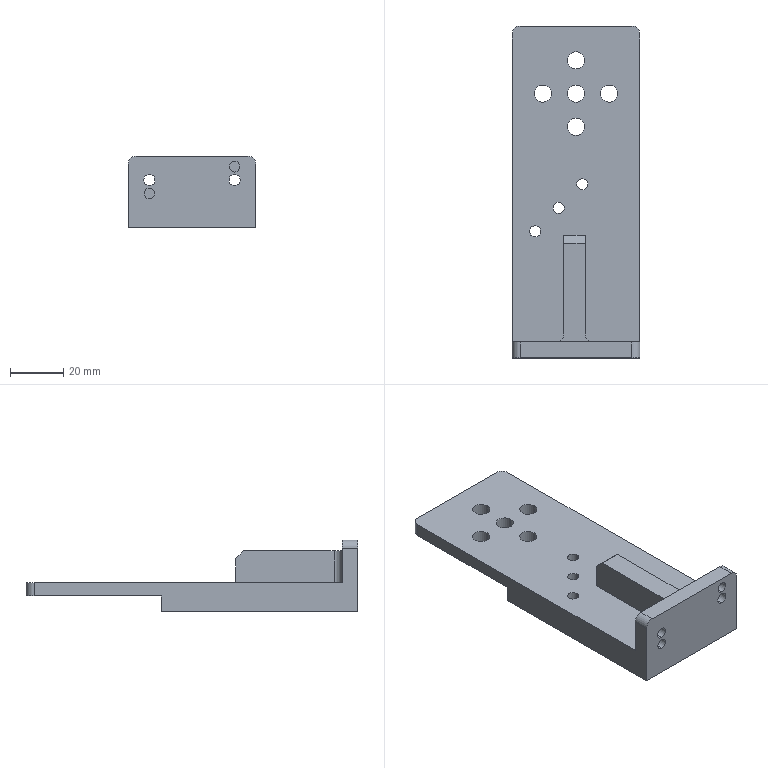NC program | NX | posted with a generic post | part box 48 x 124.7 x 27 mm
Lines 1 to 1858 of 3165, first 1663 of 1848 lines:
N10 G17 G21 G94 G90
(FLOOR_WALL_COPY_COPY , TOOL : D80)
N12 T19 M6
N14 G54
N16 G17 G0 G90 X-107.35 Y0. B0. C0. S6500 M3
N18 G43 Z30. H19
N20 Z5.
N22 G94 G1 Z2. F1500.
N24 X-102.35
N26 X102.35
N28 X107.35
N30 Z5.
N32 G0 Z30.
N34 X-107.35
N36 Z4.
N38 G1 Z1.
N40 X-102.35
N42 X102.35
N44 X107.35
N46 Z4.
N48 G0 Z30.
N50 X-107.35
N52 Z3.
N54 G1 Z0.
N56 X-102.35
N58 X102.35
N60 X107.35
N62 Z3.
N64 G0 Z30.
N66 M5
(FLOOR_WALL , TOOL : D10)
N68 T15 M6
N70 G54
N72 G17 G0 G90 X66.85 Y29.047 B0. C0. S9500 M3
N74 G43 Z30. H15
N76 Z-12.9
N78 G94 G1 Z-14.9 F1000.
N80 Y28.971 Z-15.283
N82 Y28.754 Z-15.607
N84 Y28.429 Z-15.824
N86 Y28.047 Z-15.9
N88 Y23.784
N90 Y-23.739 F3000.
N92 X66.834 Y-23.827
N94 G2 X66.446 Y-24.694 R8.
N96 G1 X66.417 Y-24.744
N98 X66.355 Y-24.729
N100 X66.352 Y-24.671
N102 Y24.805
N104 X66.373 Y24.876
N106 X66.32 Y24.927
N108 G3 X65.991 Y25.461 R8.
N110 G1 X65.942 Y25.523
N112 X65.86 Y25.498
N114 X65.854 Y25.419
N116 Y-25.578
N118 X65.87 Y-25.664
N120 X65.806 Y-25.725
N122 G2 X65.488 Y-26.131 R8.
N124 G1 X65.437 Y-26.187
N126 X65.359 Y-26.159
N128 X65.356 Y-26.083
N130 Y26.19
N132 X65.367 Y26.29
N134 X65.292 Y26.357
N136 G3 X65.028 Y26.635 R8.
N138 X64.858 Y26.565 R0.1
N140 G1 Y-26.694
N142 G2 X64.777 Y-26.877 R0.25
N144 X64.524 Y-27.101 R8.
N146 X64.359 Y-27.025 R0.1
N148 G1 Y27.117
N150 G3 X64.263 Y27.313 R0.25
N152 X64.06 Y27.467 R8.
N154 X63.861 Y27.366 R0.125
N156 G1 Y-27.473
N158 G2 X63.749 Y-27.682 R0.25
N160 X63.554 Y-27.806 R8.
N162 X63.363 Y-27.7 R0.125
N164 G1 Y27.775
N166 G3 X63.235 Y27.994 R0.25
N168 G1 X63.085 Y28.074
N170 G3 X62.865 Y27.942 R0.15
N172 G1 Y-28.029
N174 G2 X62.721 Y-28.255 R0.25
N176 G1 X62.578 Y-28.32
N178 G2 X62.367 Y-28.183 R0.15
N180 G1 Y28.239
N182 G3 X62.206 Y28.473 R0.25
N184 G1 X62.104 Y28.511
N186 G3 X61.869 Y28.347 R0.175
N188 G1 Y-28.41
N190 G2 X61.692 Y-28.649 R0.25
N192 G1 X61.595 Y-28.679
N194 G2 X61.371 Y-28.511 R0.175
N196 G1 Y28.545
N198 G3 X61.178 Y28.788 R0.25
N200 G1 X61.117 Y28.802
N202 G3 X60.873 Y28.607 R0.2
N204 G1 Y-28.645
N206 G2 X60.664 Y-28.891 R0.25
N208 G1 X60.606 Y-28.901
N210 G2 X60.375 Y-28.703 R0.2
N212 G1 Y28.711
N214 G3 X60.15 Y28.96 R0.25
N216 G1 X60.123 Y28.963
N218 G3 X59.877 Y28.739 R0.225
N220 G1 Y-28.746
N222 G2 X59.636 Y-28.995 R0.249
N224 G1 X59.611 Y-28.996
N226 G2 X59.378 Y-28.771 R0.225
N228 G1 Y28.751
N230 G3 X59.13 Y29. R0.249
N232 G1 X59.105
N234 G3 X58.88 Y28.776 R0.224
N236 G1 Y-28.776
N238 G2 X58.656 Y-29. R0.224
N240 G1 X58.632
N242 G2 X58.382 Y-28.75 R0.25
N244 G1 Y28.776
N246 G3 X58.158 Y29. R0.224
N248 G1 X58.134
N250 G3 X57.884 Y28.75 R0.25
N252 G1 Y-28.776
N254 G2 X57.66 Y-29. R0.224
N256 G1 X57.636
N258 G2 X57.386 Y-28.75 R0.25
N260 G1 Y28.776
N262 G3 X57.162 Y29. R0.224
N264 G1 X57.138
N266 G3 X56.888 Y28.75 R0.25
N268 G1 Y-28.776
N270 G2 X56.664 Y-29. R0.224
N272 G1 X56.64
N274 G2 X56.39 Y-28.75 R0.25
N276 G1 Y28.776
N278 G3 X56.166 Y29. R0.224
N280 G1 X56.142
N282 G3 X55.892 Y28.75 R0.25
N284 G1 Y-28.776
N286 G2 X55.668 Y-29. R0.224
N288 G1 X55.644
N290 G2 X55.394 Y-28.75 R0.25
N292 G1 Y28.776
N294 G3 X55.17 Y29. R0.224
N296 G1 X55.146
N298 G3 X54.896 Y28.75 R0.25
N300 G1 Y-28.776
N302 G2 X54.671 Y-29. R0.224
N304 G1 X54.647
N306 G2 X54.397 Y-28.75 R0.25
N308 G1 Y28.776
N310 G3 X54.173 Y29. R0.224
N312 G1 X54.149
N314 G3 X53.899 Y28.75 R0.25
N316 G1 Y-28.776
N318 G2 X53.675 Y-29. R0.224
N320 G1 X53.651
N322 G2 X53.401 Y-28.75 R0.25
N324 G1 Y28.776
N326 G3 X53.177 Y29. R0.224
N328 G1 X53.153
N330 G3 X52.903 Y28.75 R0.25
N332 G1 Y-28.776
N334 G2 X52.679 Y-29. R0.224
N336 G1 X52.655
N338 G2 X52.405 Y-28.75 R0.25
N340 G1 Y28.776
N342 G3 X52.181 Y29. R0.224
N344 G1 X52.157
N346 G3 X51.907 Y28.75 R0.25
N348 G1 Y-28.776
N350 G2 X51.683 Y-29. R0.224
N352 G1 X51.659
N354 G2 X51.409 Y-28.75 R0.25
N356 G1 Y28.776
N358 G3 X51.185 Y29. R0.224
N360 G1 X51.161
N362 G3 X50.911 Y28.75 R0.25
N364 G1 Y-28.776
N366 G2 X50.687 Y-29. R0.224
N368 G1 X50.663
N370 G2 X50.413 Y-28.75 R0.25
N372 G1 Y28.776
N374 G3 X50.189 Y29. R0.224
N376 G1 X50.165
N378 G3 X49.915 Y28.75 R0.25
N380 G1 Y-28.776
N382 G2 X49.69 Y-29. R0.224
N384 G1 X49.666
N386 G2 X49.416 Y-28.75 R0.25
N388 G1 Y28.776
N390 G3 X49.192 Y29. R0.224
N392 G1 X49.168
N394 G3 X48.918 Y28.75 R0.25
N396 G1 Y-28.776
N398 G2 X48.694 Y-29. R0.224
N400 G1 X48.67
N402 G2 X48.42 Y-28.75 R0.25
N404 G1 Y28.776
N406 G3 X48.196 Y29. R0.224
N408 G1 X48.172
N410 G3 X47.922 Y28.75 R0.25
N412 G1 Y-28.776
N414 G2 X47.698 Y-29. R0.224
N416 G1 X47.674
N418 G2 X47.424 Y-28.75 R0.25
N420 G1 Y28.776
N422 G3 X47.2 Y29. R0.224
N424 G1 X47.176
N426 G3 X46.926 Y28.75 R0.25
N428 G1 Y-28.776
N430 G2 X46.702 Y-29. R0.224
N432 G1 X46.678
N434 G2 X46.428 Y-28.75 R0.25
N436 G1 Y28.776
N438 G3 X46.204 Y29. R0.224
N440 G1 X46.18
N442 G3 X45.93 Y28.75 R0.25
N444 G1 Y-28.776
N446 G2 X45.706 Y-29. R0.224
N448 G1 X45.682
N450 G2 X45.432 Y-28.75 R0.25
N452 G1 Y28.776
N454 G3 X45.207 Y29. R0.224
N456 G1 X45.184
N458 G3 X44.934 Y28.75 R0.25
N460 G1 Y-28.776
N462 G2 X44.709 Y-29. R0.224
N464 G1 X44.685
N466 G2 X44.435 Y-28.75 R0.25
N468 G1 Y28.776
N470 G3 X44.211 Y29. R0.224
N472 G1 X44.187
N474 G3 X43.937 Y28.75 R0.25
N476 G1 Y-28.776
N478 G2 X43.713 Y-29. R0.224
N480 G1 X43.689
N482 G2 X43.439 Y-28.75 R0.25
N484 G1 Y28.776
N486 G3 X43.215 Y29. R0.224
N488 G1 X43.191
N490 G3 X42.941 Y28.75 R0.25
N492 G1 Y-28.776
N494 G2 X42.717 Y-29. R0.224
N496 G1 X42.693
N498 G2 X42.443 Y-28.75 R0.25
N500 G1 Y28.776
N502 G3 X42.219 Y29. R0.224
N504 G1 X42.195
N506 G3 X41.945 Y28.75 R0.25
N508 G1 Y-28.776
N510 G2 X41.721 Y-29. R0.224
N512 G1 X41.697
N514 G2 X41.447 Y-28.75 R0.25
N516 G1 Y28.776
N518 G3 X41.223 Y29. R0.224
N520 G1 X41.199
N522 G3 X40.949 Y28.75 R0.25
N524 G1 Y-28.776
N526 G2 X40.725 Y-29. R0.224
N528 G1 X40.701
N530 G2 X40.451 Y-28.75 R0.25
N532 G1 Y28.776
N534 G3 X40.226 Y29. R0.224
N536 G1 X40.203
N538 G3 X39.953 Y28.75 R0.25
N540 G1 Y-28.776
N542 G2 X39.728 Y-29. R0.224
N544 G1 X39.704
N546 G2 X39.454 Y-28.75 R0.25
N548 G1 Y28.776
N550 G3 X39.23 Y29. R0.224
N552 G1 X39.206
N554 G3 X38.956 Y28.75 R0.25
N556 G1 Y-28.776
N558 G2 X38.732 Y-29. R0.224
N560 G1 X38.708
N562 G2 X38.458 Y-28.75 R0.25
N564 G1 Y28.776
N566 G3 X38.234 Y29. R0.224
N568 G1 X38.21
N570 G3 X37.96 Y28.75 R0.25
N572 G1 Y-28.776
N574 G2 X37.736 Y-29. R0.224
N576 G1 X37.712
N578 G2 X37.462 Y-28.75 R0.25
N580 G1 Y28.776
N582 G3 X37.238 Y29. R0.224
N584 G1 X37.214
N586 G3 X36.964 Y28.75 R0.25
N588 G1 Y-28.776
N590 G2 X36.74 Y-29. R0.224
N592 G1 X36.716
N594 G2 X36.466 Y-28.75 R0.25
N596 G1 Y28.776
N598 G3 X36.242 Y29. R0.224
N600 G1 X36.218
N602 G3 X35.968 Y28.75 R0.25
N604 G1 Y-28.776
N606 G2 X35.744 Y-29. R0.224
N608 G1 X35.72
N610 G2 X35.47 Y-28.75 R0.25
N612 G1 Y28.776
N614 G3 X35.245 Y29. R0.224
N616 G1 X35.222
N618 G3 X34.972 Y28.75 R0.25
N620 G1 Y-28.776
N622 G2 X34.747 Y-29. R0.224
N624 G1 X34.723
N626 G2 X34.473 Y-28.75 R0.25
N628 G1 Y28.776
N630 G3 X34.249 Y29. R0.224
N632 G1 X34.225
N634 G3 X33.975 Y28.75 R0.25
N636 G1 Y-28.776
N638 G2 X33.751 Y-29. R0.224
N640 G1 X33.727
N642 G2 X33.477 Y-28.75 R0.25
N644 G1 Y28.776
N646 G3 X33.253 Y29. R0.224
N648 G1 X33.229
N650 G3 X32.979 Y28.75 R0.25
N652 G1 Y-28.776
N654 G2 X32.755 Y-29. R0.224
N656 G1 X32.731
N658 G2 X32.481 Y-28.75 R0.25
N660 G1 Y28.776
N662 G3 X32.257 Y29. R0.224
N664 G1 X32.233
N666 G3 X31.983 Y28.75 R0.25
N668 G1 Y-28.776
N670 G2 X31.759 Y-29. R0.224
N672 G1 X31.735
N674 G2 X31.485 Y-28.75 R0.25
N676 G1 Y28.776
N678 G3 X31.261 Y29. R0.224
N680 G1 X31.237
N682 G3 X30.987 Y28.75 R0.25
N684 G1 Y-28.776
N686 G2 X30.763 Y-29. R0.224
N688 G1 X30.739
N690 G2 X30.489 Y-28.75 R0.25
N692 G1 Y28.776
N694 G3 X30.264 Y29. R0.224
N696 G1 X30.241
N698 G3 X29.991 Y28.75 R0.25
N700 G1 Y-28.776
N702 G2 X29.766 Y-29. R0.224
N704 G1 X29.742
N706 G2 X29.492 Y-28.75 R0.25
N708 G1 Y28.776
N710 G3 X29.268 Y29. R0.224
N712 G1 X29.244
N714 G3 X28.994 Y28.75 R0.25
N716 G1 Y-28.776
N718 G2 X28.77 Y-29. R0.224
N720 G1 X28.746
N722 G2 X28.496 Y-28.75 R0.25
N724 G1 Y28.776
N726 G3 X28.272 Y29. R0.224
N728 G1 X28.248
N730 G3 X27.998 Y28.75 R0.25
N732 G1 Y-28.776
N734 G2 X27.774 Y-29. R0.224
N736 G1 X27.75
N738 G2 X27.5 Y-28.75 R0.25
N740 G1 Y28.776
N742 G3 X27.276 Y29. R0.224
N744 G1 X27.252
N746 G3 X27.002 Y28.75 R0.25
N748 G1 Y-28.776
N750 G2 X26.778 Y-29. R0.224
N752 G1 X26.754
N754 G2 X26.504 Y-28.75 R0.25
N756 G1 Y28.776
N758 G3 X26.28 Y29. R0.224
N760 G1 X26.256
N762 G3 X26.006 Y28.75 R0.25
N764 G1 Y-28.776
N766 G2 X25.782 Y-29. R0.224
N768 G1 X25.758
N770 G2 X25.508 Y-28.75 R0.25
N772 G1 Y28.776
N774 G3 X25.283 Y29. R0.224
N776 G1 X25.259
N778 G3 X25.009 Y28.75 R0.25
N780 G1 Y-28.776
N782 G2 X24.785 Y-29. R0.224
N784 G1 X24.761
N786 G2 X24.511 Y-28.75 R0.25
N788 G1 Y28.776
N790 G3 X24.287 Y29. R0.224
N792 G1 X24.263
N794 G3 X24.013 Y28.75 R0.25
N796 G1 Y-28.776
N798 G2 X23.789 Y-29. R0.224
N800 G1 X23.765
N802 G2 X23.515 Y-28.75 R0.25
N804 G1 Y28.776
N806 G3 X23.291 Y29. R0.224
N808 G1 X23.267
N810 G3 X23.017 Y28.75 R0.25
N812 G1 Y-28.776
N814 G2 X22.793 Y-29. R0.224
N816 G1 X22.769
N818 G2 X22.519 Y-28.75 R0.25
N820 G1 Y28.776
N822 G3 X22.295 Y29. R0.224
N824 G1 X22.271
N826 G3 X22.021 Y28.75 R0.25
N828 G1 Y-28.776
N830 G2 X21.797 Y-29. R0.224
N832 G1 X21.773
N834 G2 X21.523 Y-28.75 R0.25
N836 G1 Y28.776
N838 G3 X21.299 Y29. R0.224
N840 G1 X21.275
N842 G3 X21.025 Y28.75 R0.25
N844 G1 Y-28.776
N846 G2 X20.801 Y-29. R0.224
N848 G1 X20.777
N850 G2 X20.527 Y-28.75 R0.25
N852 G1 Y28.776
N854 G3 X20.302 Y29. R0.224
N856 G1 X20.278
N858 G3 X20.028 Y28.75 R0.25
N860 G1 Y-28.776
N862 G2 X19.804 Y-29. R0.224
N864 G1 X19.78
N866 G2 X19.53 Y-28.75 R0.25
N868 G1 Y28.776
N870 G3 X19.306 Y29. R0.224
N872 G1 X19.282
N874 G3 X19.032 Y28.75 R0.25
N876 G1 Y-28.776
N878 G2 X18.808 Y-29. R0.224
N880 G1 X18.784
N882 G2 X18.534 Y-28.75 R0.25
N884 G1 Y28.776
N886 G3 X18.31 Y29. R0.224
N888 G1 X18.286
N890 G3 X18.036 Y28.75 R0.25
N892 G1 Y-28.776
N894 G2 X17.812 Y-29. R0.224
N896 G1 X17.788
N898 G2 X17.538 Y-28.75 R0.25
N900 G1 Y28.776
N902 G3 X17.314 Y29. R0.224
N904 G1 X17.29
N906 G3 X17.04 Y28.75 R0.25
N908 G1 Y-28.776
N910 G2 X16.816 Y-29. R0.224
N912 G1 X16.792
N914 G2 X16.542 Y-28.75 R0.25
N916 G1 Y28.776
N918 G3 X16.318 Y29. R0.224
N920 G1 X16.294
N922 G3 X16.044 Y28.75 R0.25
N924 G1 Y-28.776
N926 G2 X15.82 Y-29. R0.224
N928 G1 X15.796
N930 G2 X15.546 Y-28.75 R0.25
N932 G1 Y28.776
N934 G3 X15.321 Y29. R0.224
N936 G1 X15.297
N938 G3 X15.047 Y28.75 R0.25
N940 G1 Y-28.776
N942 G2 X14.823 Y-29. R0.224
N944 G1 X14.799
N946 G2 X14.549 Y-28.75 R0.25
N948 G1 Y28.776
N950 G3 X14.325 Y29. R0.224
N952 G1 X14.301
N954 G3 X14.051 Y28.75 R0.25
N956 G1 Y-28.776
N958 G2 X13.827 Y-29. R0.224
N960 G1 X13.803
N962 G2 X13.553 Y-28.75 R0.25
N964 G1 Y28.776
N966 G3 X13.329 Y29. R0.224
N968 G1 X13.305
N970 G3 X13.055 Y28.75 R0.25
N972 G1 Y-28.776
N974 G2 X12.831 Y-29. R0.224
N976 G1 X12.807
N978 G2 X12.557 Y-28.75 R0.25
N980 G1 Y28.776
N982 G3 X12.333 Y29. R0.224
N984 G1 X12.309
N986 G3 X12.059 Y28.75 R0.25
N988 G1 Y-28.776
N990 G2 X11.835 Y-29. R0.224
N992 G1 X11.811
N994 G2 X11.561 Y-28.75 R0.25
N996 G1 Y28.776
N998 G3 X11.337 Y29. R0.224
N1000 G1 X11.313
N1002 G3 X11.063 Y28.75 R0.25
N1004 G1 Y-28.776
N1006 G2 X10.839 Y-29. R0.224
N1008 G1 X10.815
N1010 G2 X10.565 Y-28.75 R0.25
N1012 G1 Y28.776
N1014 G3 X10.34 Y29. R0.224
N1016 G1 X10.316
N1018 G3 X10.066 Y28.75 R0.25
N1020 G1 Y-28.776
N1022 G2 X9.842 Y-29. R0.224
N1024 G1 X9.818
N1026 G2 X9.568 Y-28.75 R0.25
N1028 G1 Y28.776
N1030 G3 X9.344 Y29. R0.224
N1032 G1 X9.32
N1034 G3 X9.07 Y28.75 R0.25
N1036 G1 Y-28.776
N1038 G2 X8.846 Y-29. R0.224
N1040 G1 X8.822
N1042 G2 X8.572 Y-28.75 R0.25
N1044 G1 Y28.776
N1046 G3 X8.348 Y29. R0.224
N1048 G1 X8.324
N1050 G3 X8.074 Y28.75 R0.25
N1052 G1 Y-28.776
N1054 G2 X7.85 Y-29. R0.224
N1056 G1 X7.826
N1058 G2 X7.576 Y-28.75 R0.25
N1060 G1 Y28.776
N1062 G3 X7.352 Y29. R0.224
N1064 G1 X7.328
N1066 G3 X7.078 Y28.75 R0.25
N1068 G1 Y-28.776
N1070 G2 X6.854 Y-29. R0.224
N1072 G1 X6.83
N1074 G2 X6.58 Y-28.75 R0.25
N1076 G1 Y28.776
N1078 G3 X6.356 Y29. R0.224
N1080 G1 X6.332
N1082 G3 X6.082 Y28.75 R0.25
N1084 G1 Y-28.776
N1086 G2 X5.858 Y-29. R0.224
N1088 G1 X5.834
N1090 G2 X5.584 Y-28.75 R0.25
N1092 G1 Y28.776
N1094 G3 X5.359 Y29. R0.224
N1096 G1 X5.335
N1098 G3 X5.085 Y28.75 R0.25
N1100 G1 Y-28.776
N1102 G2 X4.861 Y-29. R0.224
N1104 G1 X4.837
N1106 G2 X4.587 Y-28.75 R0.25
N1108 G1 Y28.776
N1110 G3 X4.363 Y29. R0.224
N1112 G1 X4.339
N1114 G3 X4.089 Y28.75 R0.25
N1116 G1 Y-28.776
N1118 G2 X3.865 Y-29. R0.224
N1120 G1 X3.841
N1122 G2 X3.591 Y-28.75 R0.25
N1124 G1 Y28.776
N1126 G3 X3.367 Y29. R0.224
N1128 G1 X3.343
N1130 G3 X3.093 Y28.75 R0.25
N1132 G1 Y-28.776
N1134 G2 X2.869 Y-29. R0.224
N1136 G1 X2.845
N1138 G2 X2.595 Y-28.75 R0.25
N1140 G1 Y28.776
N1142 G3 X2.371 Y29. R0.224
N1144 G1 X2.347
N1146 G3 X2.097 Y28.75 R0.25
N1148 G1 Y-28.776
N1150 G2 X1.873 Y-29. R0.224
N1152 G1 X1.849
N1154 G2 X1.599 Y-28.75 R0.25
N1156 G1 Y28.776
N1158 G3 X1.375 Y29. R0.224
N1160 G1 X1.351
N1162 G3 X1.101 Y28.75 R0.25
N1164 G1 Y-28.776
N1166 G2 X0.876 Y-29. R0.224
N1168 G1 X0.853
N1170 G2 X0.603 Y-28.75 R0.25
N1172 G1 Y28.776
N1174 G3 X0.378 Y29. R0.224
N1176 G1 X0.354
N1178 G3 X0.104 Y28.75 R0.25
N1180 G1 Y-28.776
N1182 G2 X-0.12 Y-29. R0.224
N1184 G1 X-0.144
N1186 G2 X-0.394 Y-28.75 R0.25
N1188 G1 Y28.776
N1190 G3 X-0.618 Y29. R0.224
N1192 G1 X-0.642
N1194 G3 X-0.892 Y28.75 R0.25
N1196 G1 Y-28.776
N1198 G2 X-1.116 Y-29. R0.224
N1200 G1 X-1.14
N1202 G2 X-1.39 Y-28.75 R0.25
N1204 G1 Y28.776
N1206 G3 X-1.614 Y29. R0.224
N1208 G1 X-1.638
N1210 G3 X-1.888 Y28.75 R0.25
N1212 G1 Y-28.776
N1214 G2 X-2.112 Y-29. R0.224
N1216 G1 X-2.136
N1218 G2 X-2.386 Y-28.75 R0.25
N1220 G1 Y28.776
N1222 G3 X-2.61 Y29. R0.224
N1224 G1 X-2.634
N1226 G3 X-2.884 Y28.75 R0.25
N1228 G1 Y-28.776
N1230 G2 X-3.108 Y-29. R0.224
N1232 G1 X-3.132
N1234 G2 X-3.382 Y-28.75 R0.25
N1236 G1 Y28.776
N1238 G3 X-3.606 Y29. R0.224
N1240 G1 X-3.63
N1242 G3 X-3.88 Y28.75 R0.25
N1244 G1 Y-28.776
N1246 G2 X-4.105 Y-29. R0.224
N1248 G1 X-4.128
N1250 G2 X-4.378 Y-28.75 R0.25
N1252 G1 Y28.776
N1254 G3 X-4.603 Y29. R0.224
N1256 G1 X-4.627
N1258 G3 X-4.877 Y28.75 R0.25
N1260 G1 Y-28.776
N1262 G2 X-5.101 Y-29. R0.224
N1264 G1 X-5.125
N1266 G2 X-5.375 Y-28.75 R0.25
N1268 G1 Y28.776
N1270 G3 X-5.599 Y29. R0.224
N1272 G1 X-5.623
N1274 G3 X-5.873 Y28.75 R0.25
N1276 G1 Y-28.776
N1278 G2 X-6.097 Y-29. R0.224
N1280 G1 X-6.121
N1282 G2 X-6.371 Y-28.75 R0.25
N1284 G1 Y28.776
N1286 G3 X-6.595 Y29. R0.224
N1288 G1 X-6.619
N1290 G3 X-6.869 Y28.75 R0.25
N1292 G1 Y-28.776
N1294 G2 X-7.093 Y-29. R0.224
N1296 G1 X-7.117
N1298 G2 X-7.367 Y-28.75 R0.25
N1300 G1 Y28.776
N1302 G3 X-7.591 Y29. R0.224
N1304 G1 X-7.615
N1306 G3 X-7.865 Y28.75 R0.25
N1308 G1 Y-28.776
N1310 G2 X-8.089 Y-29. R0.224
N1312 G1 X-8.113
N1314 G2 X-8.363 Y-28.75 R0.25
N1316 G1 Y28.776
N1318 G3 X-8.587 Y29. R0.224
N1320 G1 X-8.611
N1322 G3 X-8.861 Y28.75 R0.25
N1324 G1 Y-28.776
N1326 G2 X-9.086 Y-29. R0.224
N1328 G1 X-9.109
N1330 G2 X-9.359 Y-28.75 R0.25
N1332 G1 Y28.776
N1334 G3 X-9.584 Y29. R0.224
N1336 G1 X-9.608
N1338 G3 X-9.858 Y28.75 R0.25
N1340 G1 Y-28.776
N1342 G2 X-10.082 Y-29. R0.224
N1344 G1 X-10.106
N1346 G2 X-10.356 Y-28.75 R0.25
N1348 G1 Y28.776
N1350 G3 X-10.58 Y29. R0.224
N1352 G1 X-10.604
N1354 G3 X-10.854 Y28.75 R0.25
N1356 G1 Y-28.776
N1358 G2 X-11.078 Y-29. R0.224
N1360 G1 X-11.102
N1362 G2 X-11.352 Y-28.75 R0.25
N1364 G1 Y-8.826
N1366 G3 X-11.601 Y-8.577 R0.249
N1368 G1 X-11.626
N1370 G3 X-11.85 Y-8.801 R0.224
N1372 G1 Y-28.776
N1374 G2 X-12.074 Y-29. R0.224
N1376 G1 X-12.098
N1378 G2 X-12.348 Y-28.75 R0.25
N1380 G1 Y-8.801
N1382 G3 X-12.572 Y-8.577 R0.224
N1384 G1 X-12.596
N1386 G3 X-12.846 Y-8.827 R0.25
N1388 G1 Y-28.776
N1390 G2 X-13.07 Y-29. R0.224
N1392 G1 X-13.094
N1394 G2 X-13.344 Y-28.75 R0.25
N1396 G1 Y-8.801
N1398 G3 X-13.568 Y-8.577 R0.224
N1400 G1 X-13.592
N1402 G3 X-13.842 Y-8.827 R0.25
N1404 G1 Y-28.776
N1406 G2 X-14.067 Y-29. R0.224
N1408 G1 X-14.091
N1410 G2 X-14.341 Y-28.75 R0.25
N1412 G1 Y-8.801
N1414 G3 X-14.565 Y-8.577 R0.224
N1416 G1 X-14.589
N1418 G3 X-14.839 Y-8.827 R0.25
N1420 G1 Y-28.776
N1422 G2 X-15.063 Y-29. R0.224
N1424 G1 X-15.087
N1426 G2 X-15.337 Y-28.75 R0.25
N1428 G1 Y-8.801
N1430 G3 X-15.561 Y-8.577 R0.224
N1432 G1 X-15.585
N1434 G3 X-15.835 Y-8.827 R0.25
N1436 G1 Y-28.776
N1438 G2 X-16.059 Y-29. R0.224
N1440 G1 X-16.083
N1442 G2 X-16.333 Y-28.75 R0.25
N1444 G1 Y-8.801
N1446 G3 X-16.557 Y-8.577 R0.224
N1448 G1 X-16.581
N1450 G3 X-16.831 Y-8.827 R0.25
N1452 G1 Y-28.776
N1454 G2 X-17.055 Y-29. R0.224
N1456 G1 X-17.079
N1458 G2 X-17.329 Y-28.75 R0.25
N1460 G1 Y-8.801
N1462 G3 X-17.553 Y-8.577 R0.224
N1464 G1 X-17.577
N1466 G3 X-17.827 Y-8.827 R0.25
N1468 G1 Y-28.776
N1470 G2 X-18.051 Y-29. R0.224
N1472 G1 X-18.075
N1474 G2 X-18.325 Y-28.75 R0.25
N1476 G1 Y-8.801
N1478 G3 X-18.549 Y-8.577 R0.224
N1480 G1 X-18.573
N1482 G3 X-18.823 Y-8.827 R0.25
N1484 G1 Y-28.776
N1486 G2 X-19.048 Y-29. R0.224
N1488 G1 X-19.072
N1490 G2 X-19.322 Y-28.75 R0.25
N1492 G1 Y-8.801
N1494 G3 X-19.546 Y-8.577 R0.224
N1496 G1 X-19.57
N1498 G3 X-19.82 Y-8.827 R0.25
N1500 G1 Y-28.776
N1502 G2 X-20.044 Y-29. R0.224
N1504 G1 X-20.068
N1506 G2 X-20.318 Y-28.75 R0.25
N1508 G1 Y-8.801
N1510 G3 X-20.542 Y-8.577 R0.224
N1512 G1 X-20.566
N1514 G3 X-20.816 Y-8.827 R0.25
N1516 G1 Y-28.776
N1518 G2 X-21.04 Y-29. R0.224
N1520 G1 X-21.064
N1522 G2 X-21.314 Y-28.75 R0.25
N1524 G1 Y-8.801
N1526 G3 X-21.538 Y-8.577 R0.224
N1528 G1 X-21.562
N1530 G3 X-21.812 Y-8.827 R0.25
N1532 G1 Y-28.776
N1534 G2 X-22.036 Y-29. R0.224
N1536 G1 X-22.06
N1538 G2 X-22.31 Y-28.75 R0.25
N1540 G1 Y-8.801
N1542 G3 X-22.534 Y-8.577 R0.224
N1544 G1 X-22.558
N1546 G3 X-22.808 Y-8.827 R0.25
N1548 G1 Y-28.776
N1550 G2 X-23.032 Y-29. R0.224
N1552 G1 X-23.056
N1554 G2 X-23.306 Y-28.75 R0.25
N1556 G1 Y-8.801
N1558 G3 X-23.53 Y-8.577 R0.224
N1560 G1 X-23.554
N1562 G3 X-23.804 Y-8.827 R0.25
N1564 G1 Y-28.776
N1566 G2 X-24.029 Y-29. R0.224
N1568 G1 X-24.053
N1570 G2 X-24.303 Y-28.75 R0.25
N1572 G1 Y-8.801
N1574 G3 X-24.527 Y-8.577 R0.224
N1576 G1 X-24.551
N1578 G3 X-24.801 Y-8.827 R0.25
N1580 G1 Y-28.776
N1582 G2 X-25.025 Y-29. R0.224
N1584 G1 X-25.049
N1586 G2 X-25.299 Y-28.75 R0.25
N1588 G1 Y-8.801
N1590 G3 X-25.523 Y-8.577 R0.224
N1592 G1 X-25.547
N1594 G3 X-25.797 Y-8.827 R0.25
N1596 G1 Y-28.776
N1598 G2 X-26.021 Y-29. R0.224
N1600 G1 X-26.045
N1602 G2 X-26.295 Y-28.75 R0.25
N1604 G1 Y-8.801
N1606 G3 X-26.519 Y-8.577 R0.224
N1608 G1 X-26.543
N1610 G3 X-26.793 Y-8.827 R0.25
N1612 G1 Y-28.776
N1614 G2 X-27.017 Y-29. R0.224
N1616 G1 X-27.041
N1618 G2 X-27.291 Y-28.75 R0.25
N1620 G1 Y-8.801
N1622 G3 X-27.515 Y-8.577 R0.224
N1624 G1 X-27.539
N1626 G3 X-27.789 Y-8.827 R0.25
N1628 G1 Y-28.776
N1630 G2 X-28.013 Y-29. R0.224
N1632 G1 X-28.037
N1634 G2 X-28.287 Y-28.75 R0.25
N1636 G1 Y-8.801
N1638 G3 X-28.511 Y-8.577 R0.224
N1640 G1 X-28.535
N1642 G3 X-28.785 Y-8.827 R0.25
N1644 G1 Y-28.776
N1646 G2 X-29.01 Y-29. R0.224
N1648 G1 X-29.034
N1650 G2 X-29.284 Y-28.75 R0.25
N1652 G1 Y-8.801
N1654 G3 X-29.508 Y-8.577 R0.224
N1656 G1 X-29.532
N1658 G3 X-29.782 Y-8.827 R0.25
N1660 G1 Y-28.776
N1662 G2 X-30.006 Y-29. R0.224
N1664 G1 X-30.03
N1666 G2 X-30.28 Y-28.75 R0.25
N1668 G1 Y-8.801
N1670 G3 X-30.504 Y-8.577 R0.224
N1672 G1 X-30.528
N1674 G3 X-30.778 Y-8.827 R0.25
N1676 G1 Y-28.776
N1678 G2 X-31.002 Y-29. R0.224
N1680 G1 X-31.026
N1682 G2 X-31.276 Y-28.75 R0.25
N1684 G1 Y-8.801
N1686 G3 X-31.5 Y-8.577 R0.224
N1688 G1 X-31.524
N1690 G3 X-31.774 Y-8.827 R0.25
N1692 G1 Y-28.776
N1694 G2 X-31.998 Y-29. R0.224
N1696 G1 X-32.022
N1698 G2 X-32.272 Y-28.75 R0.25
N1700 G1 Y-8.826
N1702 G3 X-32.521 Y-8.577 R0.249
N1704 G1 X-32.546
N1706 G3 X-32.77 Y-8.801 R0.224
N1708 G1 Y-28.776
N1710 G2 X-32.994 Y-29. R0.224
N1712 G1 X-33.018
N1714 G2 X-33.268 Y-28.75 R0.25
N1716 G1 Y-8.826
N1718 G3 X-33.517 Y-8.577 R0.249
N1720 G1 X-33.542
N1722 G3 X-33.766 Y-8.801 R0.224
N1724 G1 Y-28.776
N1726 G2 X-33.991 Y-29. R0.224
N1728 G1 X-34.015
N1730 G2 X-34.265 Y-28.75 R0.25
N1732 G1 Y-8.826
N1734 G3 X-34.514 Y-8.577 R0.249
N1736 G1 X-34.539
N1738 G3 X-34.763 Y-8.801 R0.224
N1740 G1 Y-28.776
N1742 G2 X-34.987 Y-29. R0.224
N1744 G1 X-35.011
N1746 G2 X-35.261 Y-28.75 R0.25
N1748 G1 Y-8.826
N1750 G3 X-35.51 Y-8.577 R0.249
N1752 G1 X-35.535
N1754 G3 X-35.759 Y-8.801 R0.224
N1756 G1 Y-28.776
N1758 G2 X-35.983 Y-29. R0.224
N1760 G1 X-36.007
N1762 G2 X-36.257 Y-28.75 R0.25
N1764 G1 Y-8.826
N1766 G3 X-36.506 Y-8.577 R0.249
N1768 G1 X-36.531
N1770 G3 X-36.755 Y-8.801 R0.224
N1772 G1 Y-28.776
N1774 G2 X-36.979 Y-29. R0.224
N1776 G1 X-37.003
N1778 G2 X-37.253 Y-28.75 R0.25
N1780 G1 Y-8.826
N1782 G3 X-37.502 Y-8.577 R0.249
N1784 G1 X-37.527
N1786 G3 X-37.751 Y-8.801 R0.224
N1788 G1 Y-28.776
N1790 G2 X-37.975 Y-29. R0.224
N1792 G1 X-37.999
N1794 G2 X-38.249 Y-28.75 R0.25
N1796 G1 Y-8.801
N1798 G3 X-38.473 Y-8.577 R0.224
N1800 G1 X-38.497
N1802 G3 X-38.747 Y-8.827 R0.25
N1804 G1 Y-28.776
N1806 G2 X-38.972 Y-29. R0.224
N1808 G1 X-38.996
N1810 G2 X-39.246 Y-28.75 R0.25
N1812 G1 Y-8.826
N1814 G3 X-39.495 Y-8.577 R0.249
N1816 G1 X-39.52
N1818 G3 X-39.744 Y-8.801 R0.224
N1820 G1 Y-28.776
N1822 G2 X-39.968 Y-29. R0.224
N1824 G1 X-39.992
N1826 G2 X-40.242 Y-28.75 R0.25
N1828 G1 Y-8.826
N1830 G3 X-40.491 Y-8.577 R0.249
N1832 G1 X-40.516
N1834 G3 X-40.74 Y-8.801 R0.224
N1836 G1 Y-28.776
N1838 G2 X-40.964 Y-29. R0.224
N1840 G1 X-40.988
N1842 G2 X-41.238 Y-28.75 R0.25
N1844 G1 Y-8.826
N1846 G3 X-41.487 Y-8.577 R0.249
N1848 G1 X-41.512
N1850 G3 X-41.736 Y-8.801 R0.224
N1852 G1 Y-28.776
N1854 G2 X-41.96 Y-29. R0.224
N1856 G1 X-41.984
N1858 G2 X-42.234 Y-28.75 R0.25
N1860 G1 Y-8.801
N1862 G3 X-42.458 Y-8.577 R0.224
N1864 G1 X-42.482
N1866 G3 X-42.732 Y-8.827 R0.25
N1868 G1 Y-28.776
N1870 G2 X-42.956 Y-29. R0.224
N1872 G1 X-42.98
N1874 G2 X-43.23 Y-28.75 R0.25
N1876 G1 Y-8.801
N1878 G3 X-43.455 Y-8.577 R0.224
N1880 G1 X-43.478
N1882 G3 X-43.728 Y-8.827 R0.25
N1884 G1 Y-28.776
N1886 G2 X-43.953 Y-29. R0.224
N1888 G1 X-43.977
N1890 G2 X-44.227 Y-28.75 R0.25
N1892 G1 Y-8.826
N1894 G3 X-44.476 Y-8.577 R0.249
N1896 G1 X-44.501
N1898 G3 X-44.725 Y-8.801 R0.224
N1900 G1 Y-28.776
N1902 G2 X-44.949 Y-29. R0.224
N1904 G1 X-44.973
N1906 G2 X-45.223 Y-28.75 R0.25
N1908 G1 Y-8.801
N1910 G3 X-45.447 Y-8.577 R0.224
N1912 G1 X-45.471
N1914 G3 X-45.721 Y-8.827 R0.25
N1916 G1 Y-28.776
N1918 G2 X-45.945 Y-29. R0.224
N1920 G1 X-45.969
N1922 G2 X-46.219 Y-28.75 R0.25
N1924 G1 Y-8.801
N1926 G3 X-46.443 Y-8.577 R0.224
N1928 G1 X-46.467
N1930 G3 X-46.717 Y-8.827 R0.25
N1932 G1 Y-28.776
N1934 G2 X-46.941 Y-29. R0.224
N1936 G1 X-46.965
N1938 G2 X-47.215 Y-28.75 R0.25
N1940 G1 Y-8.801
N1942 G3 X-47.439 Y-8.577 R0.224
N1944 G1 X-47.463
N1946 G3 X-47.713 Y-8.827 R0.25
N1948 G1 Y-28.776
N1950 G2 X-47.937 Y-29. R0.224
N1952 G1 X-47.961
N1954 G2 X-48.211 Y-28.75 R0.25
N1956 G1 Y-8.801
N1958 G3 X-48.436 Y-8.577 R0.224
N1960 G1 X-48.459
N1962 G3 X-48.709 Y-8.827 R0.25
N1964 G1 Y-28.776
N1966 G2 X-48.934 Y-29. R0.224
N1968 G1 X-48.958
N1970 G2 X-49.208 Y-28.75 R0.25
N1972 G1 Y-8.801
N1974 G3 X-49.432 Y-8.577 R0.224
N1976 G1 X-49.456
N1978 G3 X-49.706 Y-8.827 R0.25
N1980 G1 Y-28.776
N1982 G2 X-49.93 Y-29. R0.224
N1984 G1 X-49.954
N1986 G2 X-50.204 Y-28.75 R0.25
N1988 G1 Y-8.803
N1990 G3 X-50.455 Y-8.61 R0.2
N1992 G1 X-50.536 Y-8.635
N1994 G3 X-50.702 Y-8.87 R0.25
N1996 G1 Y-28.776
N1998 G2 X-50.926 Y-29. R0.224
N2000 G1 X-50.95
N2002 G2 X-51.2 Y-28.75 R0.25
N2004 G1 Y-9.57
N2006 Z-12.9
N2008 G0 Z29.
N2010 X-51.124 Y-9.569 Z29.383
N2012 X-50.907 Y-9.563 Z29.707
N2014 X-50.583 Y-9.555 Z29.924
N2016 X-50.2 Y-9.545 Z30.
N2018 X-12.352 Y-8.602
N2020 X-11.969 Y-8.592 Z29.924
N2022 X-11.645 Y-8.584 Z29.707
N2024 X-11.428 Y-8.579 Z29.383
N2026 X-11.352 Y-8.577 Z29.
N2028 Z-12.9
N2030 G1 Z-15.824 F1000.
N2032 X-11.33 Z-15.878
N2034 X-11.276 Z-15.9
N2036 X-11.223 Y-8.593
N2038 X-11.184 Y-8.554
N2040 X-11.2 Y-8.501
N2042 Y9.647
N2044 X-11.184 Y9.7
N2046 X-11.223 Y9.739
N2048 X-11.276 Y9.723
N2050 X-11.352
N2052 Y28.776 F3000.
N2054 G3 X-11.576 Y29. R0.224
N2056 G1 X-11.6
N2058 G3 X-11.85 Y28.75 R0.25
N2060 G1 Y9.972
N2062 G2 X-12.099 Y9.723 R0.249
N2064 G1 X-12.124
N2066 G2 X-12.348 Y9.947 R0.224
N2068 G1 Y28.776
N2070 G3 X-12.572 Y29. R0.224
N2072 G1 X-12.596
N2074 G3 X-12.846 Y28.75 R0.25
N2076 G1 Y9.972
N2078 G2 X-13.095 Y9.723 R0.249
N2080 G1 X-13.12
N2082 G2 X-13.344 Y9.947 R0.224
N2084 G1 Y28.776
N2086 G3 X-13.568 Y29. R0.224
N2088 G1 X-13.592
N2090 G3 X-13.842 Y28.75 R0.25
N2092 G1 Y9.947
N2094 G2 X-14.067 Y9.723 R0.224
N2096 G1 X-14.091
N2098 G2 X-14.341 Y9.973 R0.25
N2100 G1 Y28.776
N2102 G3 X-14.565 Y29. R0.224
N2104 G1 X-14.589
N2106 G3 X-14.839 Y28.75 R0.25
N2108 G1 Y9.947
N2110 G2 X-15.063 Y9.723 R0.224
N2112 G1 X-15.087
N2114 G2 X-15.337 Y9.973 R0.25
N2116 G1 Y28.776
N2118 G3 X-15.561 Y29. R0.224
N2120 G1 X-15.585
N2122 G3 X-15.835 Y28.75 R0.25
N2124 G1 Y9.947
N2126 G2 X-16.059 Y9.723 R0.224
N2128 G1 X-16.083
N2130 G2 X-16.333 Y9.973 R0.25
N2132 G1 Y28.776
N2134 G3 X-16.557 Y29. R0.224
N2136 G1 X-16.581
N2138 G3 X-16.831 Y28.75 R0.25
N2140 G1 Y9.947
N2142 G2 X-17.055 Y9.723 R0.224
N2144 G1 X-17.079
N2146 G2 X-17.329 Y9.973 R0.25
N2148 G1 Y28.776
N2150 G3 X-17.553 Y29. R0.224
N2152 G1 X-17.577
N2154 G3 X-17.827 Y28.75 R0.25
N2156 G1 Y9.947
N2158 G2 X-18.051 Y9.723 R0.224
N2160 G1 X-18.075
N2162 G2 X-18.325 Y9.973 R0.25
N2164 G1 Y28.776
N2166 G3 X-18.549 Y29. R0.224
N2168 G1 X-18.573
N2170 G3 X-18.823 Y28.75 R0.25
N2172 G1 Y9.972
N2174 G2 X-19.072 Y9.723 R0.249
N2176 G1 X-19.097
N2178 G2 X-19.322 Y9.947 R0.224
N2180 G1 Y28.776
N2182 G3 X-19.546 Y29. R0.224
N2184 G1 X-19.57
N2186 G3 X-19.82 Y28.75 R0.25
N2188 G1 Y9.947
N2190 G2 X-20.044 Y9.723 R0.224
N2192 G1 X-20.068
N2194 G2 X-20.318 Y9.973 R0.25
N2196 G1 Y28.776
N2198 G3 X-20.542 Y29. R0.224
N2200 G1 X-20.566
N2202 G3 X-20.816 Y28.75 R0.25
N2204 G1 Y9.947
N2206 G2 X-21.04 Y9.723 R0.224
N2208 G1 X-21.064
N2210 G2 X-21.314 Y9.973 R0.25
N2212 G1 Y28.776
N2214 G3 X-21.538 Y29. R0.224
N2216 G1 X-21.562
N2218 G3 X-21.812 Y28.75 R0.25
N2220 G1 Y9.947
N2222 G2 X-22.036 Y9.723 R0.224
N2224 G1 X-22.06
N2226 G2 X-22.31 Y9.973 R0.25
N2228 G1 Y28.776
N2230 G3 X-22.534 Y29. R0.224
N2232 G1 X-22.558
N2234 G3 X-22.808 Y28.75 R0.25
N2236 G1 Y9.947
N2238 G2 X-23.032 Y9.723 R0.224
N2240 G1 X-23.056
N2242 G2 X-23.306 Y9.973 R0.25
N2244 G1 Y28.776
N2246 G3 X-23.53 Y29. R0.224
N2248 G1 X-23.554
N2250 G3 X-23.804 Y28.75 R0.25
N2252 G1 Y9.947
N2254 G2 X-24.029 Y9.723 R0.224
N2256 G1 X-24.053
N2258 G2 X-24.303 Y9.973 R0.25
N2260 G1 Y28.776
N2262 G3 X-24.527 Y29. R0.224
N2264 G1 X-24.551
N2266 G3 X-24.801 Y28.75 R0.25
N2268 G1 Y9.947
N2270 G2 X-25.025 Y9.723 R0.224
N2272 G1 X-25.049
N2274 G2 X-25.299 Y9.973 R0.25
N2276 G1 Y28.776
N2278 G3 X-25.523 Y29. R0.224
N2280 G1 X-25.547
N2282 G3 X-25.797 Y28.75 R0.25
N2284 G1 Y9.947
N2286 G2 X-26.021 Y9.723 R0.224
N2288 G1 X-26.045
N2290 G2 X-26.295 Y9.973 R0.25
N2292 G1 Y28.776
N2294 G3 X-26.519 Y29. R0.224
N2296 G1 X-26.543
N2298 G3 X-26.793 Y28.75 R0.25
N2300 G1 Y9.947
N2302 G2 X-27.017 Y9.723 R0.224
N2304 G1 X-27.041
N2306 G2 X-27.291 Y9.973 R0.25
N2308 G1 Y28.776
N2310 G3 X-27.515 Y29. R0.224
N2312 G1 X-27.539
N2314 G3 X-27.789 Y28.75 R0.25
N2316 G1 Y9.947
N2318 G2 X-28.013 Y9.723 R0.224
N2320 G1 X-28.037
N2322 G2 X-28.287 Y9.973 R0.25
N2324 G1 Y28.776
N2326 G3 X-28.511 Y29. R0.224
N2328 G1 X-28.535
N2330 G3 X-28.785 Y28.75 R0.25
N2332 G1 Y9.947
N2334 G2 X-29.01 Y9.723 R0.224
N2336 G1 X-29.034
N2338 G2 X-29.284 Y9.973 R0.25
N2340 G1 Y28.776
N2342 G3 X-29.508 Y29. R0.224
N2344 G1 X-29.532
N2346 G3 X-29.782 Y28.75 R0.25
N2348 G1 Y9.947
N2350 G2 X-30.006 Y9.723 R0.224
N2352 G1 X-30.03
N2354 G2 X-30.28 Y9.973 R0.25
N2356 G1 Y28.776
N2358 G3 X-30.504 Y29. R0.224
N2360 G1 X-30.528
N2362 G3 X-30.778 Y28.75 R0.25
N2364 G1 Y9.947
N2366 G2 X-31.002 Y9.723 R0.224
N2368 G1 X-31.026
N2370 G2 X-31.276 Y9.973 R0.25
N2372 G1 Y28.776
N2374 G3 X-31.5 Y29. R0.224
N2376 G1 X-31.524
N2378 G3 X-31.774 Y28.75 R0.25
N2380 G1 Y9.947
N2382 G2 X-31.998 Y9.723 R0.224
N2384 G1 X-32.022
N2386 G2 X-32.272 Y9.973 R0.25
N2388 G1 Y28.776
N2390 G3 X-32.496 Y29. R0.224
N2392 G1 X-32.52
N2394 G3 X-32.77 Y28.75 R0.25
N2396 G1 Y9.947
N2398 G2 X-32.994 Y9.723 R0.224
N2400 G1 X-33.018
N2402 G2 X-33.268 Y9.973 R0.25
N2404 G1 Y28.776
N2406 G3 X-33.492 Y29. R0.224
N2408 G1 X-33.516
N2410 G3 X-33.766 Y28.75 R0.25
N2412 G1 Y9.947
N2414 G2 X-33.991 Y9.723 R0.224
N2416 G1 X-34.015
N2418 G2 X-34.265 Y9.973 R0.25
N2420 G1 Y28.776
N2422 G3 X-34.489 Y29. R0.224
N2424 G1 X-34.513
N2426 G3 X-34.763 Y28.75 R0.25
N2428 G1 Y9.947
N2430 G2 X-34.987 Y9.723 R0.224
N2432 G1 X-35.011
N2434 G2 X-35.261 Y9.973 R0.25
N2436 G1 Y28.776
N2438 G3 X-35.485 Y29. R0.224
N2440 G1 X-35.509
N2442 G3 X-35.759 Y28.75 R0.25
N2444 G1 Y9.972
N2446 G2 X-36.008 Y9.723 R0.249
N2448 G1 X-36.033
N2450 G2 X-36.257 Y9.947 R0.224
N2452 G1 Y28.776
N2454 G3 X-36.481 Y29. R0.224
N2456 G1 X-36.505
N2458 G3 X-36.755 Y28.75 R0.25
N2460 G1 Y9.947
N2462 G2 X-36.979 Y9.723 R0.224
N2464 G1 X-37.003
N2466 G2 X-37.253 Y9.973 R0.25
N2468 G1 Y28.776
N2470 G3 X-37.477 Y29. R0.224
N2472 G1 X-37.501
N2474 G3 X-37.751 Y28.75 R0.25
N2476 G1 Y9.947
N2478 G2 X-37.975 Y9.723 R0.224
N2480 G1 X-37.999
N2482 G2 X-38.249 Y9.973 R0.25
N2484 G1 Y28.776
N2486 G3 X-38.473 Y29. R0.224
N2488 G1 X-38.497
N2490 G3 X-38.747 Y28.75 R0.25
N2492 G1 Y9.947
N2494 G2 X-38.972 Y9.723 R0.224
N2496 G1 X-38.996
N2498 G2 X-39.246 Y9.973 R0.25
N2500 G1 Y28.776
N2502 G3 X-39.47 Y29. R0.224
N2504 G1 X-39.494
N2506 G3 X-39.744 Y28.75 R0.25
N2508 G1 Y9.947
N2510 G2 X-39.968 Y9.723 R0.224
N2512 G1 X-39.992
N2514 G2 X-40.242 Y9.973 R0.25
N2516 G1 Y28.776
N2518 G3 X-40.466 Y29. R0.224
N2520 G1 X-40.49
N2522 G3 X-40.74 Y28.75 R0.25
N2524 G1 Y9.947
N2526 G2 X-40.964 Y9.723 R0.224
N2528 G1 X-40.988
N2530 G2 X-41.238 Y9.973 R0.25
N2532 G1 Y28.776
N2534 G3 X-41.462 Y29. R0.224
N2536 G1 X-41.486
N2538 G3 X-41.736 Y28.75 R0.25
N2540 G1 Y9.947
N2542 G2 X-41.96 Y9.723 R0.224
N2544 G1 X-41.984
N2546 G2 X-42.234 Y9.973 R0.25
N2548 G1 Y28.776
N2550 G3 X-42.458 Y29. R0.224
N2552 G1 X-42.482
N2554 G3 X-42.732 Y28.75 R0.25
N2556 G1 Y9.947
N2558 G2 X-42.956 Y9.723 R0.224
N2560 G1 X-42.98
N2562 G2 X-43.23 Y9.973 R0.25
N2564 G1 Y28.776
N2566 G3 X-43.455 Y29. R0.224
N2568 G1 X-43.478
N2570 G3 X-43.728 Y28.75 R0.25
N2572 G1 Y9.947
N2574 G2 X-43.953 Y9.723 R0.224
N2576 G1 X-43.977
N2578 G2 X-44.227 Y9.973 R0.25
N2580 G1 Y28.776
N2582 G3 X-44.451 Y29. R0.224
N2584 G1 X-44.475
N2586 G3 X-44.725 Y28.75 R0.25
N2588 G1 Y9.947
N2590 G2 X-44.949 Y9.723 R0.224
N2592 G1 X-44.973
N2594 G2 X-45.223 Y9.973 R0.25
N2596 G1 Y28.776
N2598 G3 X-45.447 Y29. R0.224
N2600 G1 X-45.471
N2602 G3 X-45.721 Y28.75 R0.25
N2604 G1 Y9.947
N2606 G2 X-45.945 Y9.723 R0.224
N2608 G1 X-45.969
N2610 G2 X-46.219 Y9.973 R0.25
N2612 G1 Y28.776
N2614 G3 X-46.443 Y29. R0.224
N2616 G1 X-46.467
N2618 G3 X-46.717 Y28.75 R0.25
N2620 G1 Y9.972
N2622 G2 X-46.966 Y9.723 R0.249
N2624 G1 X-46.991
N2626 G2 X-47.215 Y9.947 R0.224
N2628 G1 Y28.776
N2630 G3 X-47.439 Y29. R0.224
N2632 G1 X-47.463
N2634 G3 X-47.713 Y28.75 R0.25
N2636 G1 Y9.947
N2638 G2 X-47.937 Y9.723 R0.224
N2640 G1 X-47.961
N2642 G2 X-48.211 Y9.973 R0.25
N2644 G1 Y28.776
N2646 G3 X-48.436 Y29. R0.224
N2648 G1 X-48.459
N2650 G3 X-48.709 Y28.75 R0.25
N2652 G1 Y9.947
N2654 G2 X-48.934 Y9.723 R0.224
N2656 G1 X-48.958
N2658 G2 X-49.208 Y9.973 R0.25
N2660 G1 Y28.776
N2662 G3 X-49.432 Y29. R0.224
N2664 G1 X-49.456
N2666 G3 X-49.706 Y28.75 R0.25
N2668 G1 Y9.972
N2670 G2 X-49.955 Y9.723 R0.249
N2672 G1 X-49.98
N2674 G2 X-50.204 Y9.947 R0.224
N2676 G1 Y28.776
N2678 G3 X-50.428 Y29. R0.224
N2680 G1 X-50.452
N2682 G3 X-50.702 Y28.75 R0.25
N2684 G1 Y10.054
N2686 G2 X-50.869 Y9.98 R0.1
N2688 X-51.2 Y10.716 R1.
N2690 G1 Y10.717
N2692 Y29.
N2694 Y31.15
N2696 Y31.533 Z-15.824
N2698 Y31.857 Z-15.607
N2700 Y32.074 Z-15.283
N2702 Y32.15 Z-14.9
N2704 Z-12.9
N2706 G0 Z30.
(FLOOR_WALL_COPY_2 , TOOL : D10)
N2708 X-11.85 Y15.573
N2710 Z-0.9
N2712 G1 Z-2.9 F1000.
N2714 Y15.497 Z-3.283
N2716 Y15.28 Z-3.607
N2718 Y14.956 Z-3.824
N2720 Y14.573 Z-3.9
N2722 Y12.573
N2724 Y-11.203 F3000.
N2726 G2 X-12.074 Y-11.427 R0.224
N2728 G1 X-12.098
N2730 G2 X-12.348 Y-11.177 R0.25
N2732 G1 Y12.349
N2734 G3 X-12.572 Y12.573 R0.224
N2736 G1 X-12.596
N2738 G3 X-12.846 Y12.323 R0.25
N2740 G1 Y-11.203
N2742 G2 X-13.07 Y-11.427 R0.224
N2744 G1 X-13.094
N2746 G2 X-13.344 Y-11.177 R0.25
N2748 G1 Y12.349
N2750 G3 X-13.568 Y12.573 R0.224
N2752 G1 X-13.592
N2754 G3 X-13.842 Y12.323 R0.25
N2756 G1 Y-11.203
N2758 G2 X-14.067 Y-11.427 R0.224
N2760 G1 X-14.091
N2762 G2 X-14.341 Y-11.177 R0.25
N2764 G1 Y12.349
N2766 G3 X-14.565 Y12.573 R0.224
N2768 G1 X-14.589
N2770 G3 X-14.839 Y12.323 R0.25
N2772 G1 Y-11.203
N2774 G2 X-15.063 Y-11.427 R0.224
N2776 G1 X-15.087
N2778 G2 X-15.337 Y-11.177 R0.25
N2780 G1 Y12.349
N2782 G3 X-15.561 Y12.573 R0.224
N2784 G1 X-15.585
N2786 G3 X-15.835 Y12.323 R0.25
N2788 G1 Y-11.203
N2790 G2 X-16.059 Y-11.427 R0.224
N2792 G1 X-16.083
N2794 G2 X-16.333 Y-11.177 R0.25
N2796 G1 Y12.349
N2798 G3 X-16.557 Y12.573 R0.224
N2800 G1 X-16.581
N2802 G3 X-16.831 Y12.323 R0.25
N2804 G1 Y-11.203
N2806 G2 X-17.055 Y-11.427 R0.224
N2808 G1 X-17.079
N2810 G2 X-17.329 Y-11.177 R0.25
N2812 G1 Y12.349
N2814 G3 X-17.553 Y12.573 R0.224
N2816 G1 X-17.577
N2818 G3 X-17.827 Y12.323 R0.25
N2820 G1 Y-11.203
N2822 G2 X-18.051 Y-11.427 R0.224
N2824 G1 X-18.075
N2826 G2 X-18.325 Y-11.177 R0.25
N2828 G1 Y12.349
N2830 G3 X-18.549 Y12.573 R0.224
N2832 G1 X-18.573
N2834 G3 X-18.823 Y12.323 R0.25
N2836 G1 Y-11.203
N2838 G2 X-19.048 Y-11.427 R0.224
N2840 G1 X-19.072
N2842 G2 X-19.322 Y-11.177 R0.25
N2844 G1 Y12.349
N2846 G3 X-19.546 Y12.573 R0.224
N2848 G1 X-19.57
N2850 G3 X-19.82 Y12.323 R0.25
N2852 G1 Y-11.203
N2854 G2 X-20.044 Y-11.427 R0.224
N2856 G1 X-20.068
N2858 G2 X-20.318 Y-11.177 R0.25
N2860 G1 Y12.349
N2862 G3 X-20.542 Y12.573 R0.224
N2864 G1 X-20.566
N2866 G3 X-20.816 Y12.323 R0.25
N2868 G1 Y-11.203
N2870 G2 X-21.04 Y-11.427 R0.224
N2872 G1 X-21.064
N2874 G2 X-21.314 Y-11.177 R0.25
N2876 G1 Y12.349
N2878 G3 X-21.538 Y12.573 R0.224
N2880 G1 X-21.562
N2882 G3 X-21.812 Y12.323 R0.25
N2884 G1 Y-11.203
N2886 G2 X-22.036 Y-11.427 R0.224
N2888 G1 X-22.06
N2890 G2 X-22.31 Y-11.177 R0.25
N2892 G1 Y12.349
N2894 G3 X-22.534 Y12.573 R0.224
N2896 G1 X-22.558
N2898 G3 X-22.808 Y12.323 R0.25
N2900 G1 Y-11.203
N2902 G2 X-23.032 Y-11.427 R0.224
N2904 G1 X-23.056
N2906 G2 X-23.306 Y-11.177 R0.25
N2908 G1 Y12.349
N2910 G3 X-23.53 Y12.573 R0.224
N2912 G1 X-23.554
N2914 G3 X-23.804 Y12.323 R0.25
N2916 G1 Y-11.203
N2918 G2 X-24.029 Y-11.427 R0.224
N2920 G1 X-24.053
N2922 G2 X-24.303 Y-11.177 R0.25
N2924 G1 Y12.349
N2926 G3 X-24.527 Y12.573 R0.224
N2928 G1 X-24.551
N2930 G3 X-24.801 Y12.323 R0.25
N2932 G1 Y-11.203
N2934 G2 X-25.025 Y-11.427 R0.224
N2936 G1 X-25.049
N2938 G2 X-25.299 Y-11.177 R0.25
N2940 G1 Y12.349
N2942 G3 X-25.523 Y12.573 R0.224
N2944 G1 X-25.547
N2946 G3 X-25.797 Y12.323 R0.25
N2948 G1 Y-11.203
N2950 G2 X-26.021 Y-11.427 R0.224
N2952 G1 X-26.045
N2954 G2 X-26.295 Y-11.177 R0.25
N2956 G1 Y12.349
N2958 G3 X-26.519 Y12.573 R0.224
N2960 G1 X-26.543
N2962 G3 X-26.793 Y12.323 R0.25
N2964 G1 Y-11.203
N2966 G2 X-27.017 Y-11.427 R0.224
N2968 G1 X-27.041
N2970 G2 X-27.291 Y-11.177 R0.25
N2972 G1 Y12.349
N2974 G3 X-27.515 Y12.573 R0.224
N2976 G1 X-27.539
N2978 G3 X-27.789 Y12.323 R0.25
N2980 G1 Y-11.203
N2982 G2 X-28.013 Y-11.427 R0.224
N2984 G1 X-28.037
N2986 G2 X-28.287 Y-11.177 R0.25
N2988 G1 Y12.349
N2990 G3 X-28.511 Y12.573 R0.224
N2992 G1 X-28.535
N2994 G3 X-28.785 Y12.323 R0.25
N2996 G1 Y-11.203
N2998 G2 X-29.01 Y-11.427 R0.224
N3000 G1 X-29.034
N3002 G2 X-29.284 Y-11.177 R0.25
N3004 G1 Y12.349
N3006 G3 X-29.508 Y12.573 R0.224
N3008 G1 X-29.532
N3010 G3 X-29.782 Y12.323 R0.25
N3012 G1 Y-11.203
N3014 G2 X-30.006 Y-11.427 R0.224
N3016 G1 X-30.03
N3018 G2 X-30.28 Y-11.177 R0.25
N3020 G1 Y12.349
N3022 G3 X-30.504 Y12.573 R0.224
N3024 G1 X-30.528
N3026 G3 X-30.778 Y12.323 R0.25
N3028 G1 Y-11.203
N3030 G2 X-31.002 Y-11.427 R0.224
N3032 G1 X-31.026
N3034 G2 X-31.276 Y-11.177 R0.25
N3036 G1 Y12.349
N3038 G3 X-31.5 Y12.573 R0.224
N3040 G1 X-31.524
N3042 G3 X-31.774 Y12.323 R0.25
N3044 G1 Y-11.203
N3046 G2 X-31.998 Y-11.427 R0.224
N3048 G1 X-32.022
N3050 G2 X-32.272 Y-11.177 R0.25
N3052 G1 Y12.349
N3054 G3 X-32.496 Y12.573 R0.224
N3056 G1 X-32.52
N3058 G3 X-32.77 Y12.323 R0.25
N3060 G1 Y-11.203
N3062 G2 X-32.994 Y-11.427 R0.224
N3064 G1 X-33.018
N3066 G2 X-33.268 Y-11.177 R0.25
N3068 G1 Y12.349
N3070 G3 X-33.493 Y12.573 R0.224
N3072 G1 X-33.516
N3074 G3 X-33.766 Y12.323 R0.25
N3076 G1 Y-11.203
N3078 G2 X-33.991 Y-11.427 R0.224
N3080 G1 X-34.015
N3082 G2 X-34.265 Y-11.177 R0.25
N3084 G1 Y12.349
N3086 G3 X-34.489 Y12.573 R0.224
N3088 G1 X-34.513
N3090 G3 X-34.763 Y12.323 R0.25
N3092 G1 Y-11.203
N3094 G2 X-34.987 Y-11.427 R0.224
N3096 G1 X-35.011
N3098 G2 X-35.261 Y-11.177 R0.25
N3100 G1 Y12.349
N3102 G3 X-35.485 Y12.573 R0.224
N3104 G1 X-35.509
N3106 G3 X-35.759 Y12.323 R0.25
N3108 G1 Y-11.203
N3110 G2 X-35.983 Y-11.427 R0.224
N3112 G1 X-36.007
N3114 G2 X-36.257 Y-11.177 R0.25
N3116 G1 Y12.349
N3118 G3 X-36.481 Y12.573 R0.224
N3120 G1 X-36.505
N3122 G3 X-36.755 Y12.323 R0.25
N3124 G1 Y-11.203
N3126 G2 X-36.979 Y-11.427 R0.224
N3128 G1 X-37.003
N3130 G2 X-37.253 Y-11.177 R0.25
N3132 G1 Y12.349
N3134 G3 X-37.477 Y12.573 R0.224
N3136 G1 X-37.501
N3138 G3 X-37.751 Y12.323 R0.25
N3140 G1 Y-11.203
N3142 G2 X-37.975 Y-11.427 R0.224
N3144 G1 X-37.999
N3146 G2 X-38.249 Y-11.177 R0.25
N3148 G1 Y12.349
N3150 G3 X-38.474 Y12.573 R0.224
N3152 G1 X-38.497
N3154 G3 X-38.747 Y12.323 R0.25
N3156 G1 Y-11.203
N3158 G2 X-38.972 Y-11.427 R0.224
N3160 G1 X-38.996
N3162 G2 X-39.246 Y-11.177 R0.25
N3164 G1 Y12.349
N3166 G3 X-39.47 Y12.573 R0.224
N3168 G1 X-39.494
N3170 G3 X-39.744 Y12.323 R0.25
N3172 G1 Y-11.203
N3174 G2 X-39.968 Y-11.427 R0.224
N3176 G1 X-39.992
N3178 G2 X-40.242 Y-11.177 R0.25
N3180 G1 Y12.349
N3182 G3 X-40.466 Y12.573 R0.224
N3184 G1 X-40.49
N3186 G3 X-40.74 Y12.323 R0.25
N3188 G1 Y-11.203
N3190 G2 X-40.964 Y-11.427 R0.224
N3192 G1 X-40.988
N3194 G2 X-41.238 Y-11.177 R0.25
N3196 G1 Y12.349
N3198 G3 X-41.462 Y12.573 R0.224
N3200 G1 X-41.486
N3202 G3 X-41.736 Y12.323 R0.25
N3204 G1 Y-11.203
N3206 G2 X-41.96 Y-11.427 R0.224
N3208 G1 X-41.984
N3210 G2 X-42.234 Y-11.177 R0.25
N3212 G1 Y12.349
N3214 G3 X-42.458 Y12.573 R0.224
N3216 G1 X-42.482
N3218 G3 X-42.732 Y12.323 R0.25
N3220 G1 Y-11.203
N3222 G2 X-42.956 Y-11.427 R0.224
N3224 G1 X-42.98
N3226 G2 X-43.23 Y-11.177 R0.25
N3228 G1 Y12.349
N3230 G3 X-43.455 Y12.573 R0.224
N3232 G1 X-43.478
N3234 G3 X-43.728 Y12.323 R0.25
N3236 G1 Y-11.203
N3238 G2 X-43.953 Y-11.427 R0.224
N3240 G1 X-43.977
N3242 G2 X-44.227 Y-11.177 R0.25
N3244 G1 Y12.349
N3246 G3 X-44.451 Y12.573 R0.224
N3248 G1 X-44.475
N3250 G3 X-44.725 Y12.323 R0.25
N3252 G1 Y-11.203
N3254 G2 X-44.949 Y-11.427 R0.224
N3256 G1 X-44.973
N3258 G2 X-45.223 Y-11.177 R0.25
N3260 G1 Y12.349
N3262 G3 X-45.447 Y12.573 R0.224
N3264 G1 X-45.471
N3266 G3 X-45.721 Y12.323 R0.25
N3268 G1 Y-11.203
N3270 G2 X-45.945 Y-11.427 R0.224
N3272 G1 X-45.969
N3274 G2 X-46.219 Y-11.177 R0.25
N3276 G1 Y12.349
N3278 G3 X-46.443 Y12.573 R0.224
N3280 G1 X-46.467
N3282 G3 X-46.717 Y12.323 R0.25
N3284 G1 Y-11.203
N3286 G2 X-46.941 Y-11.427 R0.224
N3288 G1 X-46.965
N3290 G2 X-47.215 Y-11.177 R0.25
N3292 G1 Y12.349
N3294 G3 X-47.439 Y12.573 R0.224
N3296 G1 X-47.463
N3298 G3 X-47.713 Y12.323 R0.25
N3300 G1 Y-11.203
N3302 G2 X-47.937 Y-11.427 R0.224
N3304 G1 X-47.961
N3306 G2 X-48.211 Y-11.177 R0.25
N3308 G1 Y12.568
N3310 X-48.212 Y12.579
N3312 X-48.342 Y15.406
N3314 G3 X-48.517 Y15.573 R0.175
N3316 G1 X-48.535
N3318 G3 X-48.709 Y15.398 R0.175
N3320 G1 Y-14.203
N3322 G2 X-48.934 Y-14.427 R0.224
N3324 G1 X-48.958
N3326 G2 X-49.208 Y-14.177 R0.25
N3328 G1 Y15.349